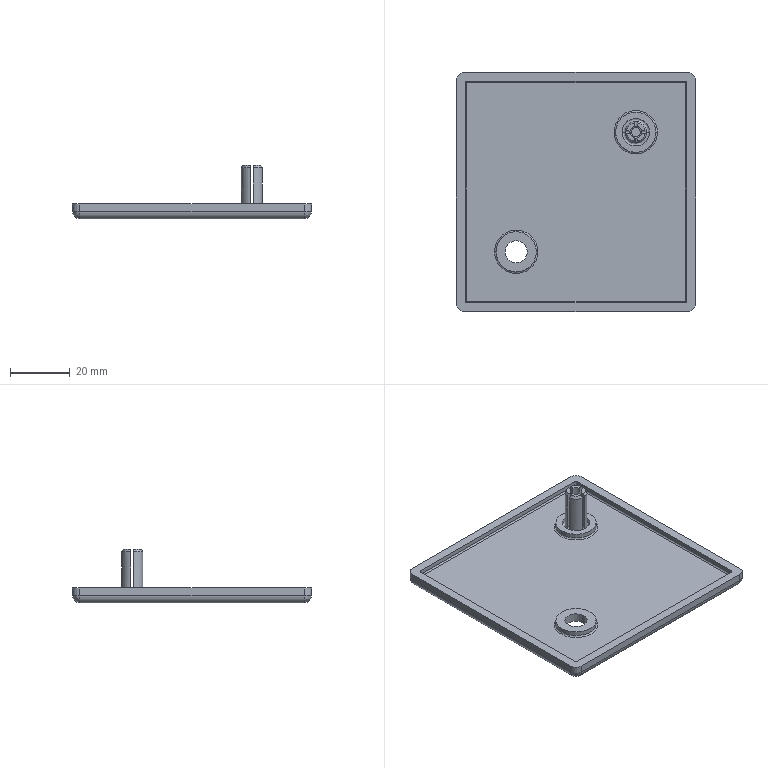Part | STEP file | 00369089_KAPPE_ABDECK_IPM-AN-8-80X80 | 1 solid | 88 faces | box 80 x 80 x 18 mm | volume 20980 mm3 | cylinder 37 | plane 31 | spline 16 | cone 4 | commonest cylinder face diameters 1 x13 5 x8 2 x4 13.5 x4 4 x2 7.2 x2